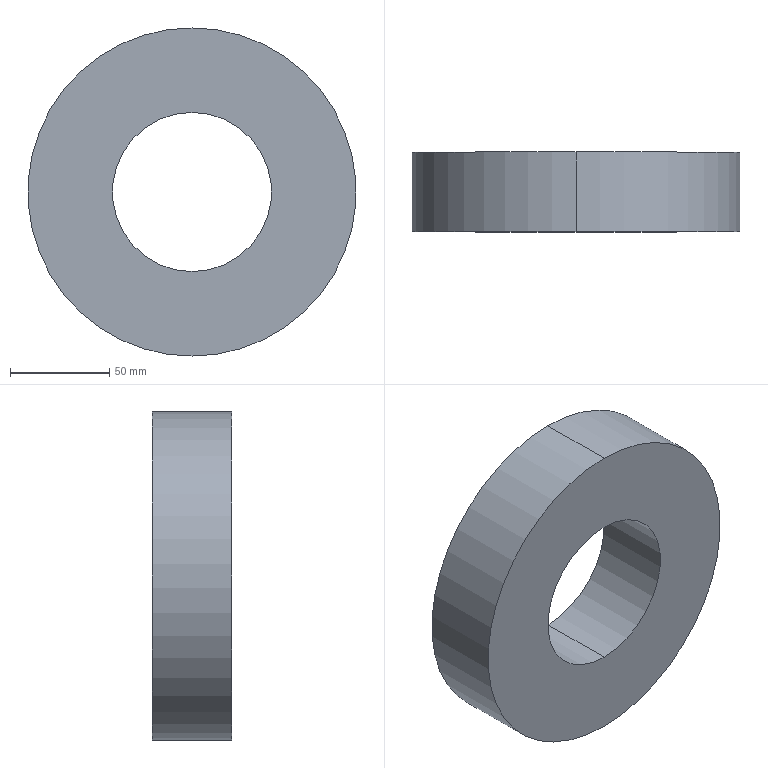Part | SolidWorks | features BaseBody 1 | 1 solid | 6 faces | box 165 x 40 x 165 mm | volume 654237 mm3 | cylinder 4 | plane 2 | commonest cylinder face diameters 80 x2 165 x2
STEP:
#1=CARTESIAN_POINT('',(0.,40.,40.));
#2=VERTEX_POINT('',#1);
#3=CARTESIAN_POINT('',(0.,40.,-40.));
#4=VERTEX_POINT('',#3);
#5=CARTESIAN_POINT('',(0.,40.,0.));
#6=DIRECTION('',(0.,-1.,0.));
#7=DIRECTION('',(0.,0.,-1.));
#8=AXIS2_PLACEMENT_3D('',#5,#6,#7);
#9=CIRCLE('',#8,40.);
#10=EDGE_CURVE('',#2,#4,#9,.T.);
#11=ORIENTED_EDGE('',*,*,#10,.F.);
#12=CARTESIAN_POINT('',(0.,0.,40.));
#13=VERTEX_POINT('',#12);
#14=CARTESIAN_POINT('',(0.,40.,40.));
#15=DIRECTION('',(0.,-1.,0.));
#16=VECTOR('',#15,1000.);
#17=LINE('',#14,#16);
#18=EDGE_CURVE('',#2,#13,#17,.T.);
#19=ORIENTED_EDGE('',*,*,#18,.T.);
#20=CARTESIAN_POINT('',(0.,0.,-40.));
#21=VERTEX_POINT('',#20);
#22=CARTESIAN_POINT('',(0.,0.,0.));
#23=DIRECTION('',(0.,1.,0.));
#24=DIRECTION('',(0.,0.,-1.));
#25=AXIS2_PLACEMENT_3D('',#22,#23,#24);
#26=CIRCLE('',#25,40.);
#27=EDGE_CURVE('',#21,#13,#26,.T.);
#28=ORIENTED_EDGE('',*,*,#27,.F.);
#29=CARTESIAN_POINT('',(0.,40.,-40.));
#30=DIRECTION('',(0.,-1.,0.));
#31=VECTOR('',#30,1000.);
#32=LINE('',#29,#31);
#33=EDGE_CURVE('',#4,#21,#32,.T.);
#34=ORIENTED_EDGE('',*,*,#33,.F.);
#35=EDGE_LOOP('',(#11,#19,#28,#34));
#36=FACE_OUTER_BOUND('',#35,.T.);
#37=CARTESIAN_POINT('',(0.,40.,0.));
#38=DIRECTION('',(0.,-1.,0.));
#39=DIRECTION('',(0.,0.,-1.));
#40=AXIS2_PLACEMENT_3D('',#37,#38,#39);
#41=CYLINDRICAL_SURFACE('',#40,40.);
#42=ADVANCED_FACE('',(#36),#41,.F.);
#43=CARTESIAN_POINT('',(0.,40.,82.5));
#44=VERTEX_POINT('',#43);
#45=CARTESIAN_POINT('',(0.,40.,-82.5));
#46=VERTEX_POINT('',#45);
#47=CARTESIAN_POINT('',(0.,40.,0.));
#48=DIRECTION('',(0.,1.,0.));
#49=DIRECTION('',(0.,0.,-1.));
#50=AXIS2_PLACEMENT_3D('',#47,#48,#49);
#51=CIRCLE('',#50,82.5);
#52=EDGE_CURVE('',#44,#46,#51,.T.);
#53=ORIENTED_EDGE('',*,*,#52,.F.);
#54=CARTESIAN_POINT('',(0.,0.,82.5));
#55=VERTEX_POINT('',#54);
#56=CARTESIAN_POINT('',(0.,40.,82.5));
#57=DIRECTION('',(0.,-1.,0.));
#58=VECTOR('',#57,1000.);
#59=LINE('',#56,#58);
#60=EDGE_CURVE('',#44,#55,#59,.T.);
#61=ORIENTED_EDGE('',*,*,#60,.T.);
#62=CARTESIAN_POINT('',(0.,0.,-82.5));
#63=VERTEX_POINT('',#62);
#64=CARTESIAN_POINT('',(0.,0.,0.));
#65=DIRECTION('',(0.,1.,0.));
#66=DIRECTION('',(0.,0.,-1.));
#67=AXIS2_PLACEMENT_3D('',#64,#65,#66);
#68=CIRCLE('',#67,82.5);
#69=EDGE_CURVE('',#55,#63,#68,.T.);
#70=ORIENTED_EDGE('',*,*,#69,.T.);
#71=CARTESIAN_POINT('',(0.,40.,-82.5));
#72=DIRECTION('',(0.,-1.,0.));
#73=VECTOR('',#72,1000.);
#74=LINE('',#71,#73);
#75=EDGE_CURVE('',#46,#63,#74,.T.);
#76=ORIENTED_EDGE('',*,*,#75,.F.);
#77=EDGE_LOOP('',(#53,#61,#70,#76));
#78=FACE_OUTER_BOUND('',#77,.T.);
#79=CARTESIAN_POINT('',(0.,40.,0.));
#80=DIRECTION('',(0.,-1.,0.));
#81=DIRECTION('',(0.,0.,-1.));
#82=AXIS2_PLACEMENT_3D('',#79,#80,#81);
#83=CYLINDRICAL_SURFACE('',#82,82.5);
#84=ADVANCED_FACE('',(#78),#83,.T.);
#85=CARTESIAN_POINT('',(0.,40.,0.));
#86=DIRECTION('',(0.,-1.,0.));
#87=DIRECTION('',(0.,0.,-1.));
#88=AXIS2_PLACEMENT_3D('',#85,#86,#87);
#89=CIRCLE('',#88,40.);
#90=EDGE_CURVE('',#4,#2,#89,.T.);
#91=ORIENTED_EDGE('',*,*,#90,.T.);
#92=ORIENTED_EDGE('',*,*,#10,.T.);
#93=EDGE_LOOP('',(#91,#92));
#94=FACE_BOUND('',#93,.T.);
#95=CARTESIAN_POINT('',(0.,40.,0.));
#96=DIRECTION('',(0.,1.,0.));
#97=DIRECTION('',(0.,0.,-1.));
#98=AXIS2_PLACEMENT_3D('',#95,#96,#97);
#99=CIRCLE('',#98,82.5);
#100=EDGE_CURVE('',#46,#44,#99,.T.);
#101=ORIENTED_EDGE('',*,*,#100,.T.);
#102=ORIENTED_EDGE('',*,*,#52,.T.);
#103=EDGE_LOOP('',(#101,#102));
#104=FACE_OUTER_BOUND('',#103,.T.);
#105=CARTESIAN_POINT('',(0.,40.,0.));
#106=DIRECTION('',(0.,1.,0.));
#107=DIRECTION('',(0.,0.,1.));
#108=AXIS2_PLACEMENT_3D('',#105,#106,#107);
#109=PLANE('',#108);
#110=ADVANCED_FACE('',(#94,#104),#109,.T.);
#111=ORIENTED_EDGE('',*,*,#18,.F.);
#112=ORIENTED_EDGE('',*,*,#90,.F.);
#113=ORIENTED_EDGE('',*,*,#33,.T.);
#114=CARTESIAN_POINT('',(0.,0.,0.));
#115=DIRECTION('',(0.,1.,0.));
#116=DIRECTION('',(0.,0.,-1.));
#117=AXIS2_PLACEMENT_3D('',#114,#115,#116);
#118=CIRCLE('',#117,40.);
#119=EDGE_CURVE('',#13,#21,#118,.T.);
#120=ORIENTED_EDGE('',*,*,#119,.F.);
#121=EDGE_LOOP('',(#111,#112,#113,#120));
#122=FACE_OUTER_BOUND('',#121,.T.);
#123=CARTESIAN_POINT('',(0.,40.,0.));
#124=DIRECTION('',(0.,-1.,0.));
#125=DIRECTION('',(0.,0.,-1.));
#126=AXIS2_PLACEMENT_3D('',#123,#124,#125);
#127=CYLINDRICAL_SURFACE('',#126,40.);
#128=ADVANCED_FACE('',(#122),#127,.F.);
#129=ORIENTED_EDGE('',*,*,#60,.F.);
#130=ORIENTED_EDGE('',*,*,#100,.F.);
#131=ORIENTED_EDGE('',*,*,#75,.T.);
#132=CARTESIAN_POINT('',(0.,0.,0.));
#133=DIRECTION('',(0.,1.,0.));
#134=DIRECTION('',(0.,0.,-1.));
#135=AXIS2_PLACEMENT_3D('',#132,#133,#134);
#136=CIRCLE('',#135,82.5);
#137=EDGE_CURVE('',#63,#55,#136,.T.);
#138=ORIENTED_EDGE('',*,*,#137,.T.);
#139=EDGE_LOOP('',(#129,#130,#131,#138));
#140=FACE_OUTER_BOUND('',#139,.T.);
#141=CARTESIAN_POINT('',(0.,40.,0.));
#142=DIRECTION('',(0.,-1.,0.));
#143=DIRECTION('',(0.,0.,-1.));
#144=AXIS2_PLACEMENT_3D('',#141,#142,#143);
#145=CYLINDRICAL_SURFACE('',#144,82.5);
#146=ADVANCED_FACE('',(#140),#145,.T.);
#147=ORIENTED_EDGE('',*,*,#27,.T.);
#148=ORIENTED_EDGE('',*,*,#119,.T.);
#149=EDGE_LOOP('',(#147,#148));
#150=FACE_BOUND('',#149,.T.);
#151=ORIENTED_EDGE('',*,*,#137,.F.);
#152=ORIENTED_EDGE('',*,*,#69,.F.);
#153=EDGE_LOOP('',(#151,#152));
#154=FACE_OUTER_BOUND('',#153,.T.);
#155=CARTESIAN_POINT('',(0.,0.,0.));
#156=DIRECTION('',(0.,1.,0.));
#157=DIRECTION('',(0.,0.,1.));
#158=AXIS2_PLACEMENT_3D('',#155,#156,#157);
#159=PLANE('',#158);
#160=ADVANCED_FACE('',(#150,#154),#159,.F.);
#161=CLOSED_SHELL('',(#42,#84,#110,#128,#146,#160));
#162=MANIFOLD_SOLID_BREP('',#161);
#163=CARTESIAN_POINT('',(0.,0.,0.));
#164=DIRECTION('',(0.,0.,1.));
#165=DIRECTION('',(1.,0.,0.));
#166=AXIS2_PLACEMENT_3D('',#163,#164,#165);
#167=(LENGTH_UNIT()NAMED_UNIT(*)SI_UNIT(.MILLI.,.METRE.));
#168=UNCERTAINTY_MEASURE_WITH_UNIT(LENGTH_MEASURE(0.00001),#167,'','');
#169=(NAMED_UNIT(*)PLANE_ANGLE_UNIT()SI_UNIT($,.RADIAN.));
#170=(NAMED_UNIT(*)SI_UNIT($,.STERADIAN.)SOLID_ANGLE_UNIT());
#171=(GEOMETRIC_REPRESENTATION_CONTEXT(3)GLOBAL_UNCERTAINTY_ASSIGNED_CONTEXT((#168))GLOBAL_UNIT_ASSIGNED_CONTEXT((#167,#169,#170))REPRESENTATION_CONTEXT('',''));
#172=ADVANCED_BREP_SHAPE_REPRESENTATION('',(#162,#166),#171);